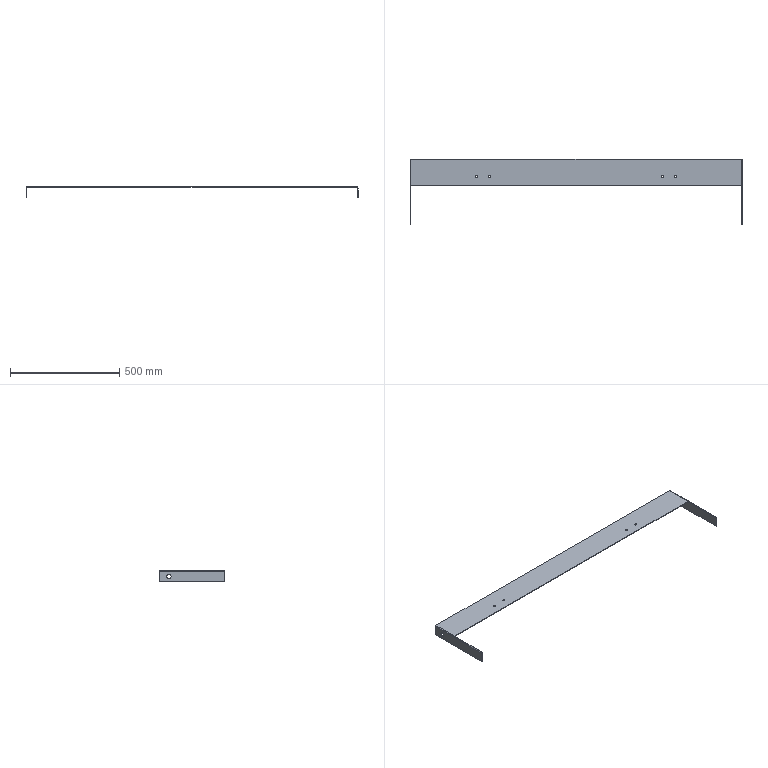Part | SolidWorks | features ICE 6, EdgeFlange 2, FlatPattern 1, MirrorPattern 1, SMBaseFlange 1, SheetMetal 1 | 1 solid | 36 faces | box 1518 x 301 x 50 mm | volume 631038 mm3 | plane 20 | cylinder 16 | commonest cylinder face diameters 9 x8 20 x4 1.473 x2 7.473 x2
STEP:
#1=CARTESIAN_POINT('',(450.763,220.,-3.));
#2=VERTEX_POINT('',#1);
#3=CARTESIAN_POINT('',(459.763,220.,-3.));
#4=VERTEX_POINT('',#3);
#5=CARTESIAN_POINT('',(455.263,220.,-3.));
#6=DIRECTION('',(0.,0.,1.));
#7=DIRECTION('',(-1.,0.,0.));
#8=AXIS2_PLACEMENT_3D('',#5,#6,#7);
#9=CIRCLE('',#8,4.5);
#10=EDGE_CURVE('',#2,#4,#9,.T.);
#11=ORIENTED_EDGE('',*,*,#10,.F.);
#12=CARTESIAN_POINT('',(450.763,220.,0.));
#13=VERTEX_POINT('',#12);
#14=CARTESIAN_POINT('',(450.763,220.,-50.));
#15=DIRECTION('',(0.,0.,1.));
#16=VECTOR('',#15,1000.);
#17=LINE('',#14,#16);
#18=EDGE_CURVE('',#2,#13,#17,.T.);
#19=ORIENTED_EDGE('',*,*,#18,.T.);
#20=CARTESIAN_POINT('',(459.763,220.,0.));
#21=VERTEX_POINT('',#20);
#22=CARTESIAN_POINT('',(455.263,220.,0.));
#23=DIRECTION('',(0.,0.,-1.));
#24=DIRECTION('',(-1.,0.,0.));
#25=AXIS2_PLACEMENT_3D('',#22,#23,#24);
#26=CIRCLE('',#25,4.5);
#27=EDGE_CURVE('',#21,#13,#26,.T.);
#28=ORIENTED_EDGE('',*,*,#27,.F.);
#29=CARTESIAN_POINT('',(459.763,220.,-50.));
#30=DIRECTION('',(0.,0.,1.));
#31=VECTOR('',#30,1000.);
#32=LINE('',#29,#31);
#33=EDGE_CURVE('',#4,#21,#32,.T.);
#34=ORIENTED_EDGE('',*,*,#33,.F.);
#35=EDGE_LOOP('',(#11,#19,#28,#34));
#36=FACE_OUTER_BOUND('',#35,.T.);
#37=CARTESIAN_POINT('',(455.263,220.,-50.));
#38=DIRECTION('',(0.,0.,1.));
#39=DIRECTION('',(1.,0.,0.));
#40=AXIS2_PLACEMENT_3D('',#37,#38,#39);
#41=CYLINDRICAL_SURFACE('',#40,4.5);
#42=ADVANCED_FACE('',(#36),#41,.F.);
#43=CARTESIAN_POINT('',(390.763,220.,-3.));
#44=VERTEX_POINT('',#43);
#45=CARTESIAN_POINT('',(399.763,220.,-3.));
#46=VERTEX_POINT('',#45);
#47=CARTESIAN_POINT('',(395.263,220.,-3.));
#48=DIRECTION('',(0.,0.,1.));
#49=DIRECTION('',(-1.,0.,0.));
#50=AXIS2_PLACEMENT_3D('',#47,#48,#49);
#51=CIRCLE('',#50,4.5);
#52=EDGE_CURVE('',#44,#46,#51,.T.);
#53=ORIENTED_EDGE('',*,*,#52,.F.);
#54=CARTESIAN_POINT('',(390.763,220.,0.));
#55=VERTEX_POINT('',#54);
#56=CARTESIAN_POINT('',(390.763,220.,-50.));
#57=DIRECTION('',(0.,0.,1.));
#58=VECTOR('',#57,1000.);
#59=LINE('',#56,#58);
#60=EDGE_CURVE('',#44,#55,#59,.T.);
#61=ORIENTED_EDGE('',*,*,#60,.T.);
#62=CARTESIAN_POINT('',(399.763,220.,0.));
#63=VERTEX_POINT('',#62);
#64=CARTESIAN_POINT('',(395.263,220.,0.));
#65=DIRECTION('',(0.,0.,1.));
#66=DIRECTION('',(-1.,0.,0.));
#67=AXIS2_PLACEMENT_3D('',#64,#65,#66);
#68=CIRCLE('',#67,4.5);
#69=EDGE_CURVE('',#55,#63,#68,.T.);
#70=ORIENTED_EDGE('',*,*,#69,.T.);
#71=CARTESIAN_POINT('',(399.763,220.,-50.));
#72=DIRECTION('',(0.,0.,1.));
#73=VECTOR('',#72,1000.);
#74=LINE('',#71,#73);
#75=EDGE_CURVE('',#46,#63,#74,.T.);
#76=ORIENTED_EDGE('',*,*,#75,.F.);
#77=EDGE_LOOP('',(#53,#61,#70,#76));
#78=FACE_OUTER_BOUND('',#77,.T.);
#79=CARTESIAN_POINT('',(395.263,220.,-50.));
#80=DIRECTION('',(0.,0.,1.));
#81=DIRECTION('',(1.,0.,0.));
#82=AXIS2_PLACEMENT_3D('',#79,#80,#81);
#83=CYLINDRICAL_SURFACE('',#82,4.5);
#84=ADVANCED_FACE('',(#78),#83,.F.);
#85=CARTESIAN_POINT('',(-450.763,220.,-3.));
#86=VERTEX_POINT('',#85);
#87=CARTESIAN_POINT('',(-459.763,220.,-3.));
#88=VERTEX_POINT('',#87);
#89=CARTESIAN_POINT('',(-455.263,220.,-3.));
#90=DIRECTION('',(0.,0.,-1.));
#91=DIRECTION('',(-1.,0.,0.));
#92=AXIS2_PLACEMENT_3D('',#89,#90,#91);
#93=CIRCLE('',#92,4.5);
#94=EDGE_CURVE('',#86,#88,#93,.T.);
#95=ORIENTED_EDGE('',*,*,#94,.T.);
#96=CARTESIAN_POINT('',(-459.763,220.,0.));
#97=VERTEX_POINT('',#96);
#98=CARTESIAN_POINT('',(-459.763,220.,-50.));
#99=DIRECTION('',(0.,0.,1.));
#100=VECTOR('',#99,1000.);
#101=LINE('',#98,#100);
#102=EDGE_CURVE('',#88,#97,#101,.T.);
#103=ORIENTED_EDGE('',*,*,#102,.T.);
#104=CARTESIAN_POINT('',(-450.763,220.,0.));
#105=VERTEX_POINT('',#104);
#106=CARTESIAN_POINT('',(-455.263,220.,0.));
#107=DIRECTION('',(0.,0.,1.));
#108=DIRECTION('',(1.,0.,0.));
#109=AXIS2_PLACEMENT_3D('',#106,#107,#108);
#110=CIRCLE('',#109,4.5);
#111=EDGE_CURVE('',#97,#105,#110,.T.);
#112=ORIENTED_EDGE('',*,*,#111,.T.);
#113=CARTESIAN_POINT('',(-450.763,220.,-50.));
#114=DIRECTION('',(0.,0.,1.));
#115=VECTOR('',#114,1000.);
#116=LINE('',#113,#115);
#117=EDGE_CURVE('',#86,#105,#116,.T.);
#118=ORIENTED_EDGE('',*,*,#117,.F.);
#119=EDGE_LOOP('',(#95,#103,#112,#118));
#120=FACE_OUTER_BOUND('',#119,.T.);
#121=CARTESIAN_POINT('',(-455.263,220.,-50.));
#122=DIRECTION('',(0.,0.,1.));
#123=DIRECTION('',(1.,0.,0.));
#124=AXIS2_PLACEMENT_3D('',#121,#122,#123);
#125=CYLINDRICAL_SURFACE('',#124,4.5);
#126=ADVANCED_FACE('',(#120),#125,.F.);
#127=CARTESIAN_POINT('',(-390.763,220.,-3.));
#128=VERTEX_POINT('',#127);
#129=CARTESIAN_POINT('',(-399.763,220.,-3.));
#130=VERTEX_POINT('',#129);
#131=CARTESIAN_POINT('',(-395.263,220.,-3.));
#132=DIRECTION('',(0.,0.,-1.));
#133=DIRECTION('',(-1.,0.,0.));
#134=AXIS2_PLACEMENT_3D('',#131,#132,#133);
#135=CIRCLE('',#134,4.5);
#136=EDGE_CURVE('',#128,#130,#135,.T.);
#137=ORIENTED_EDGE('',*,*,#136,.T.);
#138=CARTESIAN_POINT('',(-399.763,220.,0.));
#139=VERTEX_POINT('',#138);
#140=CARTESIAN_POINT('',(-399.763,220.,-50.));
#141=DIRECTION('',(0.,0.,1.));
#142=VECTOR('',#141,1000.);
#143=LINE('',#140,#142);
#144=EDGE_CURVE('',#130,#139,#143,.T.);
#145=ORIENTED_EDGE('',*,*,#144,.T.);
#146=CARTESIAN_POINT('',(-390.763,220.,0.));
#147=VERTEX_POINT('',#146);
#148=CARTESIAN_POINT('',(-395.263,220.,0.));
#149=DIRECTION('',(0.,0.,-1.));
#150=DIRECTION('',(-1.,0.,0.));
#151=AXIS2_PLACEMENT_3D('',#148,#149,#150);
#152=CIRCLE('',#151,4.5);
#153=EDGE_CURVE('',#147,#139,#152,.T.);
#154=ORIENTED_EDGE('',*,*,#153,.F.);
#155=CARTESIAN_POINT('',(-390.763,220.,-50.));
#156=DIRECTION('',(0.,0.,1.));
#157=VECTOR('',#156,1000.);
#158=LINE('',#155,#157);
#159=EDGE_CURVE('',#128,#147,#158,.T.);
#160=ORIENTED_EDGE('',*,*,#159,.F.);
#161=EDGE_LOOP('',(#137,#145,#154,#160));
#162=FACE_OUTER_BOUND('',#161,.T.);
#163=CARTESIAN_POINT('',(-395.263,220.,-50.));
#164=DIRECTION('',(0.,0.,1.));
#165=DIRECTION('',(1.,0.,0.));
#166=AXIS2_PLACEMENT_3D('',#163,#164,#165);
#167=CYLINDRICAL_SURFACE('',#166,4.5);
#168=ADVANCED_FACE('',(#162),#167,.F.);
#169=CARTESIAN_POINT('',(-759.,255.,-16.868));
#170=VERTEX_POINT('',#169);
#171=CARTESIAN_POINT('',(-759.,255.,-36.868));
#172=VERTEX_POINT('',#171);
#173=CARTESIAN_POINT('',(-759.,255.,-26.868));
#174=DIRECTION('',(1.,0.,0.));
#175=DIRECTION('',(0.,0.,-1.));
#176=AXIS2_PLACEMENT_3D('',#173,#174,#175);
#177=CIRCLE('',#176,10.);
#178=EDGE_CURVE('',#170,#172,#177,.T.);
#179=ORIENTED_EDGE('',*,*,#178,.F.);
#180=CARTESIAN_POINT('',(-756.,255.,-16.868));
#181=VERTEX_POINT('',#180);
#182=CARTESIAN_POINT('',(-759.,255.,-16.868));
#183=DIRECTION('',(1.,0.,0.));
#184=VECTOR('',#183,1000.);
#185=LINE('',#182,#184);
#186=EDGE_CURVE('',#170,#181,#185,.T.);
#187=ORIENTED_EDGE('',*,*,#186,.T.);
#188=CARTESIAN_POINT('',(-756.,255.,-36.868));
#189=VERTEX_POINT('',#188);
#190=CARTESIAN_POINT('',(-756.,255.,-26.868));
#191=DIRECTION('',(-1.,0.,0.));
#192=DIRECTION('',(0.,0.,1.));
#193=AXIS2_PLACEMENT_3D('',#190,#191,#192);
#194=CIRCLE('',#193,10.);
#195=EDGE_CURVE('',#189,#181,#194,.T.);
#196=ORIENTED_EDGE('',*,*,#195,.F.);
#197=CARTESIAN_POINT('',(-759.,255.,-36.868));
#198=DIRECTION('',(1.,0.,0.));
#199=VECTOR('',#198,1000.);
#200=LINE('',#197,#199);
#201=EDGE_CURVE('',#172,#189,#200,.T.);
#202=ORIENTED_EDGE('',*,*,#201,.F.);
#203=EDGE_LOOP('',(#179,#187,#196,#202));
#204=FACE_OUTER_BOUND('',#203,.T.);
#205=CARTESIAN_POINT('',(-759.,255.,-26.868));
#206=DIRECTION('',(1.,0.,0.));
#207=DIRECTION('',(0.,0.,-1.));
#208=AXIS2_PLACEMENT_3D('',#205,#206,#207);
#209=CYLINDRICAL_SURFACE('',#208,10.);
#210=ADVANCED_FACE('',(#204),#209,.F.);
#211=CARTESIAN_POINT('',(756.,255.,-16.868));
#212=VERTEX_POINT('',#211);
#213=CARTESIAN_POINT('',(756.,255.,-36.868));
#214=VERTEX_POINT('',#213);
#215=CARTESIAN_POINT('',(756.,255.,-26.868));
#216=DIRECTION('',(1.,0.,0.));
#217=DIRECTION('',(0.,0.,-1.));
#218=AXIS2_PLACEMENT_3D('',#215,#216,#217);
#219=CIRCLE('',#218,10.);
#220=EDGE_CURVE('',#212,#214,#219,.T.);
#221=ORIENTED_EDGE('',*,*,#220,.F.);
#222=CARTESIAN_POINT('',(759.,255.,-16.868));
#223=VERTEX_POINT('',#222);
#224=CARTESIAN_POINT('',(-759.,255.,-16.868));
#225=DIRECTION('',(1.,0.,0.));
#226=VECTOR('',#225,1000.);
#227=LINE('',#224,#226);
#228=EDGE_CURVE('',#212,#223,#227,.T.);
#229=ORIENTED_EDGE('',*,*,#228,.T.);
#230=CARTESIAN_POINT('',(759.,255.,-36.868));
#231=VERTEX_POINT('',#230);
#232=CARTESIAN_POINT('',(759.,255.,-26.868));
#233=DIRECTION('',(1.,0.,0.));
#234=DIRECTION('',(0.,0.,-1.));
#235=AXIS2_PLACEMENT_3D('',#232,#233,#234);
#236=CIRCLE('',#235,10.);
#237=EDGE_CURVE('',#223,#231,#236,.T.);
#238=ORIENTED_EDGE('',*,*,#237,.T.);
#239=CARTESIAN_POINT('',(-759.,255.,-36.868));
#240=DIRECTION('',(1.,0.,0.));
#241=VECTOR('',#240,1000.);
#242=LINE('',#239,#241);
#243=EDGE_CURVE('',#214,#231,#242,.T.);
#244=ORIENTED_EDGE('',*,*,#243,.F.);
#245=EDGE_LOOP('',(#221,#229,#238,#244));
#246=FACE_OUTER_BOUND('',#245,.T.);
#247=CARTESIAN_POINT('',(-759.,255.,-26.868));
#248=DIRECTION('',(1.,0.,0.));
#249=DIRECTION('',(0.,0.,-1.));
#250=AXIS2_PLACEMENT_3D('',#247,#248,#249);
#251=CYLINDRICAL_SURFACE('',#250,10.);
#252=ADVANCED_FACE('',(#246),#251,.F.);
#253=CARTESIAN_POINT('',(-756.,-1.,-3.737));
#254=VERTEX_POINT('',#253);
#255=CARTESIAN_POINT('',(-756.,-1.,-50.));
#256=VERTEX_POINT('',#255);
#257=CARTESIAN_POINT('',(-756.,-1.,0.));
#258=DIRECTION('',(0.,0.,-1.));
#259=VECTOR('',#258,1000.);
#260=LINE('',#257,#259);
#261=EDGE_CURVE('',#254,#256,#260,.T.);
#262=ORIENTED_EDGE('',*,*,#261,.F.);
#263=CARTESIAN_POINT('',(-759.,-1.,-3.737));
#264=VERTEX_POINT('',#263);
#265=CARTESIAN_POINT('',(-756.,-1.,-3.737));
#266=DIRECTION('',(-1.,0.,0.));
#267=VECTOR('',#266,1000.);
#268=LINE('',#265,#267);
#269=EDGE_CURVE('',#254,#264,#268,.T.);
#270=ORIENTED_EDGE('',*,*,#269,.T.);
#271=CARTESIAN_POINT('',(-759.,-1.,-50.));
#272=VERTEX_POINT('',#271);
#273=CARTESIAN_POINT('',(-759.,-1.,-141.819));
#274=DIRECTION('',(0.,0.,1.));
#275=VECTOR('',#274,1000.);
#276=LINE('',#273,#275);
#277=EDGE_CURVE('',#272,#264,#276,.T.);
#278=ORIENTED_EDGE('',*,*,#277,.F.);
#279=CARTESIAN_POINT('',(-759.,-1.,-50.));
#280=DIRECTION('',(1.,0.,0.));
#281=VECTOR('',#280,1000.);
#282=LINE('',#279,#281);
#283=EDGE_CURVE('',#272,#256,#282,.T.);
#284=ORIENTED_EDGE('',*,*,#283,.T.);
#285=EDGE_LOOP('',(#262,#270,#278,#284));
#286=FACE_OUTER_BOUND('',#285,.T.);
#287=CARTESIAN_POINT('',(-759.,-1.,-141.819));
#288=DIRECTION('',(0.,1.,0.));
#289=DIRECTION('',(0.,0.,1.));
#290=AXIS2_PLACEMENT_3D('',#287,#288,#289);
#291=PLANE('',#290);
#292=ADVANCED_FACE('',(#286),#291,.F.);
#293=CARTESIAN_POINT('',(759.,-1.,-50.));
#294=VERTEX_POINT('',#293);
#295=CARTESIAN_POINT('',(759.,-1.,-3.737));
#296=VERTEX_POINT('',#295);
#297=CARTESIAN_POINT('',(759.,-1.,0.));
#298=DIRECTION('',(0.,0.,1.));
#299=VECTOR('',#298,1000.);
#300=LINE('',#297,#299);
#301=EDGE_CURVE('',#294,#296,#300,.T.);
#302=ORIENTED_EDGE('',*,*,#301,.T.);
#303=CARTESIAN_POINT('',(756.,-1.,-3.737));
#304=VERTEX_POINT('',#303);
#305=CARTESIAN_POINT('',(759.,-1.,-3.737));
#306=DIRECTION('',(-1.,0.,0.));
#307=VECTOR('',#306,1000.);
#308=LINE('',#305,#307);
#309=EDGE_CURVE('',#296,#304,#308,.T.);
#310=ORIENTED_EDGE('',*,*,#309,.T.);
#311=CARTESIAN_POINT('',(756.,-1.,-50.));
#312=VERTEX_POINT('',#311);
#313=CARTESIAN_POINT('',(756.,-1.,0.));
#314=DIRECTION('',(0.,0.,1.));
#315=VECTOR('',#314,1000.);
#316=LINE('',#313,#315);
#317=EDGE_CURVE('',#312,#304,#316,.T.);
#318=ORIENTED_EDGE('',*,*,#317,.F.);
#319=CARTESIAN_POINT('',(759.,-1.,-50.));
#320=DIRECTION('',(1.,0.,0.));
#321=VECTOR('',#320,1000.);
#322=LINE('',#319,#321);
#323=EDGE_CURVE('',#312,#294,#322,.T.);
#324=ORIENTED_EDGE('',*,*,#323,.T.);
#325=EDGE_LOOP('',(#302,#310,#318,#324));
#326=FACE_OUTER_BOUND('',#325,.T.);
#327=CARTESIAN_POINT('',(-759.,-1.,-141.819));
#328=DIRECTION('',(0.,1.,0.));
#329=DIRECTION('',(0.,0.,1.));
#330=AXIS2_PLACEMENT_3D('',#327,#328,#329);
#331=PLANE('',#330);
#332=ADVANCED_FACE('',(#326),#331,.F.);
#333=CARTESIAN_POINT('',(455.263,220.,-3.));
#334=DIRECTION('',(0.,0.,1.));
#335=DIRECTION('',(-1.,0.,0.));
#336=AXIS2_PLACEMENT_3D('',#333,#334,#335);
#337=CIRCLE('',#336,4.5);
#338=EDGE_CURVE('',#4,#2,#337,.T.);
#339=ORIENTED_EDGE('',*,*,#338,.T.);
#340=ORIENTED_EDGE('',*,*,#10,.T.);
#341=EDGE_LOOP('',(#339,#340));
#342=FACE_BOUND('',#341,.T.);
#343=CARTESIAN_POINT('',(395.263,220.,-3.));
#344=DIRECTION('',(0.,0.,1.));
#345=DIRECTION('',(-1.,0.,0.));
#346=AXIS2_PLACEMENT_3D('',#343,#344,#345);
#347=CIRCLE('',#346,4.5);
#348=EDGE_CURVE('',#46,#44,#347,.T.);
#349=ORIENTED_EDGE('',*,*,#348,.T.);
#350=ORIENTED_EDGE('',*,*,#52,.T.);
#351=EDGE_LOOP('',(#349,#350));
#352=FACE_BOUND('',#351,.T.);
#353=ORIENTED_EDGE('',*,*,#94,.F.);
#354=CARTESIAN_POINT('',(-455.263,220.,-3.));
#355=DIRECTION('',(0.,0.,-1.));
#356=DIRECTION('',(-1.,0.,0.));
#357=AXIS2_PLACEMENT_3D('',#354,#355,#356);
#358=CIRCLE('',#357,4.5);
#359=EDGE_CURVE('',#88,#86,#358,.T.);
#360=ORIENTED_EDGE('',*,*,#359,.F.);
#361=EDGE_LOOP('',(#353,#360));
#362=FACE_BOUND('',#361,.T.);
#363=ORIENTED_EDGE('',*,*,#136,.F.);
#364=CARTESIAN_POINT('',(-395.263,220.,-3.));
#365=DIRECTION('',(0.,0.,-1.));
#366=DIRECTION('',(-1.,0.,0.));
#367=AXIS2_PLACEMENT_3D('',#364,#365,#366);
#368=CIRCLE('',#367,4.5);
#369=EDGE_CURVE('',#130,#128,#368,.T.);
#370=ORIENTED_EDGE('',*,*,#369,.F.);
#371=EDGE_LOOP('',(#363,#370));
#372=FACE_BOUND('',#371,.T.);
#373=CARTESIAN_POINT('',(-755.263,180.,-3.));
#374=VERTEX_POINT('',#373);
#375=CARTESIAN_POINT('',(755.263,180.,-3.));
#376=VERTEX_POINT('',#375);
#377=CARTESIAN_POINT('',(755.263,180.,-3.));
#378=DIRECTION('',(1.,0.,0.));
#379=VECTOR('',#378,1000.);
#380=LINE('',#377,#379);
#381=EDGE_CURVE('',#374,#376,#380,.T.);
#382=ORIENTED_EDGE('',*,*,#381,.F.);
#383=CARTESIAN_POINT('',(-755.263,300.,-3.));
#384=VERTEX_POINT('',#383);
#385=CARTESIAN_POINT('',(-755.263,300.,-3.));
#386=DIRECTION('',(0.,-1.,0.));
#387=VECTOR('',#386,1000.);
#388=LINE('',#385,#387);
#389=EDGE_CURVE('',#384,#374,#388,.T.);
#390=ORIENTED_EDGE('',*,*,#389,.F.);
#391=CARTESIAN_POINT('',(755.263,300.,-3.));
#392=VERTEX_POINT('',#391);
#393=CARTESIAN_POINT('',(-759.,300.,-3.));
#394=DIRECTION('',(-1.,0.,0.));
#395=VECTOR('',#394,1000.);
#396=LINE('',#393,#395);
#397=EDGE_CURVE('',#392,#384,#396,.T.);
#398=ORIENTED_EDGE('',*,*,#397,.F.);
#399=CARTESIAN_POINT('',(755.263,-300.,-3.));
#400=DIRECTION('',(0.,1.,0.));
#401=VECTOR('',#400,1000.);
#402=LINE('',#399,#401);
#403=EDGE_CURVE('',#376,#392,#402,.T.);
#404=ORIENTED_EDGE('',*,*,#403,.F.);
#405=EDGE_LOOP('',(#382,#390,#398,#404));
#406=FACE_OUTER_BOUND('',#405,.T.);
#407=CARTESIAN_POINT('',(0.,0.,-3.));
#408=DIRECTION('',(0.,0.,-1.));
#409=DIRECTION('',(-1.,0.,0.));
#410=AXIS2_PLACEMENT_3D('',#407,#408,#409);
#411=PLANE('',#410);
#412=ADVANCED_FACE('',(#342,#352,#362,#372,#406),#411,.T.);
#413=ORIENTED_EDGE('',*,*,#27,.T.);
#414=CARTESIAN_POINT('',(455.263,220.,0.));
#415=DIRECTION('',(0.,0.,-1.));
#416=DIRECTION('',(-1.,0.,0.));
#417=AXIS2_PLACEMENT_3D('',#414,#415,#416);
#418=CIRCLE('',#417,4.5);
#419=EDGE_CURVE('',#13,#21,#418,.T.);
#420=ORIENTED_EDGE('',*,*,#419,.T.);
#421=EDGE_LOOP('',(#413,#420));
#422=FACE_BOUND('',#421,.T.);
#423=CARTESIAN_POINT('',(395.263,220.,0.));
#424=DIRECTION('',(0.,0.,1.));
#425=DIRECTION('',(-1.,0.,0.));
#426=AXIS2_PLACEMENT_3D('',#423,#424,#425);
#427=CIRCLE('',#426,4.5);
#428=EDGE_CURVE('',#63,#55,#427,.T.);
#429=ORIENTED_EDGE('',*,*,#428,.F.);
#430=ORIENTED_EDGE('',*,*,#69,.F.);
#431=EDGE_LOOP('',(#429,#430));
#432=FACE_BOUND('',#431,.T.);
#433=CARTESIAN_POINT('',(-455.263,220.,0.));
#434=DIRECTION('',(0.,0.,1.));
#435=DIRECTION('',(1.,0.,0.));
#436=AXIS2_PLACEMENT_3D('',#433,#434,#435);
#437=CIRCLE('',#436,4.5);
#438=EDGE_CURVE('',#105,#97,#437,.T.);
#439=ORIENTED_EDGE('',*,*,#438,.F.);
#440=ORIENTED_EDGE('',*,*,#111,.F.);
#441=EDGE_LOOP('',(#439,#440));
#442=FACE_BOUND('',#441,.T.);
#443=ORIENTED_EDGE('',*,*,#153,.T.);
#444=CARTESIAN_POINT('',(-395.263,220.,0.));
#445=DIRECTION('',(0.,0.,-1.));
#446=DIRECTION('',(-1.,0.,0.));
#447=AXIS2_PLACEMENT_3D('',#444,#445,#446);
#448=CIRCLE('',#447,4.5);
#449=EDGE_CURVE('',#139,#147,#448,.T.);
#450=ORIENTED_EDGE('',*,*,#449,.T.);
#451=EDGE_LOOP('',(#443,#450));
#452=FACE_BOUND('',#451,.T.);
#453=CARTESIAN_POINT('',(-755.263,300.,0.));
#454=VERTEX_POINT('',#453);
#455=CARTESIAN_POINT('',(-755.263,180.,0.));
#456=VERTEX_POINT('',#455);
#457=CARTESIAN_POINT('',(-755.263,300.,0.));
#458=DIRECTION('',(0.,-1.,0.));
#459=VECTOR('',#458,1000.);
#460=LINE('',#457,#459);
#461=EDGE_CURVE('',#454,#456,#460,.T.);
#462=ORIENTED_EDGE('',*,*,#461,.T.);
#463=CARTESIAN_POINT('',(755.263,180.,0.));
#464=VERTEX_POINT('',#463);
#465=CARTESIAN_POINT('',(755.263,180.,0.));
#466=DIRECTION('',(1.,0.,0.));
#467=VECTOR('',#466,1000.);
#468=LINE('',#465,#467);
#469=EDGE_CURVE('',#456,#464,#468,.T.);
#470=ORIENTED_EDGE('',*,*,#469,.T.);
#471=CARTESIAN_POINT('',(755.263,300.,0.));
#472=VERTEX_POINT('',#471);
#473=CARTESIAN_POINT('',(755.263,-300.,0.));
#474=DIRECTION('',(0.,1.,0.));
#475=VECTOR('',#474,1000.);
#476=LINE('',#473,#475);
#477=EDGE_CURVE('',#464,#472,#476,.T.);
#478=ORIENTED_EDGE('',*,*,#477,.T.);
#479=CARTESIAN_POINT('',(-759.,300.,0.));
#480=DIRECTION('',(-1.,0.,0.));
#481=VECTOR('',#480,1000.);
#482=LINE('',#479,#481);
#483=EDGE_CURVE('',#472,#454,#482,.T.);
#484=ORIENTED_EDGE('',*,*,#483,.T.);
#485=EDGE_LOOP('',(#462,#470,#478,#484));
#486=FACE_OUTER_BOUND('',#485,.T.);
#487=CARTESIAN_POINT('',(0.,0.,0.));
#488=DIRECTION('',(0.,0.,-1.));
#489=DIRECTION('',(-1.,0.,0.));
#490=AXIS2_PLACEMENT_3D('',#487,#488,#489);
#491=PLANE('',#490);
#492=ADVANCED_FACE('',(#422,#432,#442,#452,#486),#491,.F.);
#493=CARTESIAN_POINT('',(755.263,300.,-3.));
#494=DIRECTION('',(0.,0.,1.));
#495=VECTOR('',#494,1000.);
#496=LINE('',#493,#495);
#497=EDGE_CURVE('',#392,#472,#496,.T.);
#498=ORIENTED_EDGE('',*,*,#497,.F.);
#499=ORIENTED_EDGE('',*,*,#397,.T.);
#500=CARTESIAN_POINT('',(-755.263,300.,-3.));
#501=DIRECTION('',(0.,0.,1.));
#502=VECTOR('',#501,1000.);
#503=LINE('',#500,#502);
#504=EDGE_CURVE('',#384,#454,#503,.T.);
#505=ORIENTED_EDGE('',*,*,#504,.T.);
#506=ORIENTED_EDGE('',*,*,#483,.F.);
#507=EDGE_LOOP('',(#498,#499,#505,#506));
#508=FACE_OUTER_BOUND('',#507,.T.);
#509=CARTESIAN_POINT('',(-759.,300.,-3.));
#510=DIRECTION('',(0.,1.,0.));
#511=DIRECTION('',(0.,0.,1.));
#512=AXIS2_PLACEMENT_3D('',#509,#510,#511);
#513=PLANE('',#512);
#514=ADVANCED_FACE('',(#508),#513,.T.);
#515=CARTESIAN_POINT('',(-756.,300.,-3.737));
#516=VERTEX_POINT('',#515);
#517=CARTESIAN_POINT('',(-755.263,300.,-3.737));
#518=DIRECTION('',(0.,1.,0.));
#519=DIRECTION('',(0.,0.,1.));
#520=AXIS2_PLACEMENT_3D('',#517,#518,#519);
#521=CIRCLE('',#520,0.7366);
#522=EDGE_CURVE('',#516,#384,#521,.T.);
#523=ORIENTED_EDGE('',*,*,#522,.F.);
#524=CARTESIAN_POINT('',(-759.,300.,-3.737));
#525=VERTEX_POINT('',#524);
#526=CARTESIAN_POINT('',(-756.,300.,-3.737));
#527=DIRECTION('',(-1.,0.,0.));
#528=VECTOR('',#527,1000.);
#529=LINE('',#526,#528);
#530=EDGE_CURVE('',#516,#525,#529,.T.);
#531=ORIENTED_EDGE('',*,*,#530,.T.);
#532=CARTESIAN_POINT('',(-755.263,300.,-3.737));
#533=DIRECTION('',(0.,1.,0.));
#534=DIRECTION('',(0.,0.,1.));
#535=AXIS2_PLACEMENT_3D('',#532,#533,#534);
#536=CIRCLE('',#535,3.737);
#537=EDGE_CURVE('',#525,#454,#536,.T.);
#538=ORIENTED_EDGE('',*,*,#537,.T.);
#539=ORIENTED_EDGE('',*,*,#504,.F.);
#540=EDGE_LOOP('',(#523,#531,#538,#539));
#541=FACE_OUTER_BOUND('',#540,.T.);
#542=CARTESIAN_POINT('',(-755.263,300.,-3.737));
#543=DIRECTION('',(0.,-1.,0.));
#544=DIRECTION('',(0.,0.,-1.));
#545=AXIS2_PLACEMENT_3D('',#542,#543,#544);
#546=PLANE('',#545);
#547=ADVANCED_FACE('',(#541),#546,.F.);
#548=CARTESIAN_POINT('',(-755.263,-1.,0.));
#549=VERTEX_POINT('',#548);
#550=CARTESIAN_POINT('',(-755.263,-1.,-3.737));
#551=DIRECTION('',(0.,-1.,0.));
#552=DIRECTION('',(0.,0.,1.));
#553=AXIS2_PLACEMENT_3D('',#550,#551,#552);
#554=CIRCLE('',#553,3.737);
#555=EDGE_CURVE('',#549,#264,#554,.T.);
#556=ORIENTED_EDGE('',*,*,#555,.F.);
#557=CARTESIAN_POINT('',(-755.263,300.,0.));
#558=DIRECTION('',(0.,-1.,0.));
#559=VECTOR('',#558,1000.);
#560=LINE('',#557,#559);
#561=EDGE_CURVE('',#456,#549,#560,.T.);
#562=ORIENTED_EDGE('',*,*,#561,.F.);
#563=ORIENTED_EDGE('',*,*,#461,.F.);
#564=ORIENTED_EDGE('',*,*,#537,.F.);
#565=CARTESIAN_POINT('',(-759.,0.,-3.737));
#566=DIRECTION('',(0.,1.,0.));
#567=VECTOR('',#566,1000.);
#568=LINE('',#565,#567);
#569=EDGE_CURVE('',#264,#525,#568,.T.);
#570=ORIENTED_EDGE('',*,*,#569,.F.);
#571=EDGE_LOOP('',(#556,#562,#563,#564,#570));
#572=FACE_OUTER_BOUND('',#571,.T.);
#573=CARTESIAN_POINT('',(-755.263,300.,-3.737));
#574=DIRECTION('',(0.,1.,0.));
#575=DIRECTION('',(-1.,0.,0.));
#576=AXIS2_PLACEMENT_3D('',#573,#574,#575);
#577=CYLINDRICAL_SURFACE('',#576,3.737);
#578=ADVANCED_FACE('',(#572),#577,.T.);
#579=CARTESIAN_POINT('',(-755.263,-1.,-3.));
#580=VERTEX_POINT('',#579);
#581=CARTESIAN_POINT('',(-755.263,300.,-3.));
#582=DIRECTION('',(0.,-1.,0.));
#583=VECTOR('',#582,1000.);
#584=LINE('',#581,#583);
#585=EDGE_CURVE('',#374,#580,#584,.T.);
#586=ORIENTED_EDGE('',*,*,#585,.T.);
#587=CARTESIAN_POINT('',(-755.263,-1.,-3.737));
#588=DIRECTION('',(0.,-1.,0.));
#589=DIRECTION('',(0.,0.,1.));
#590=AXIS2_PLACEMENT_3D('',#587,#588,#589);
#591=CIRCLE('',#590,0.7366);
#592=EDGE_CURVE('',#580,#254,#591,.T.);
#593=ORIENTED_EDGE('',*,*,#592,.T.);
#594=CARTESIAN_POINT('',(-756.,-300.,-3.737));
#595=DIRECTION('',(0.,1.,0.));
#596=VECTOR('',#595,1000.);
#597=LINE('',#594,#596);
#598=EDGE_CURVE('',#254,#516,#597,.T.);
#599=ORIENTED_EDGE('',*,*,#598,.T.);
#600=ORIENTED_EDGE('',*,*,#522,.T.);
#601=ORIENTED_EDGE('',*,*,#389,.T.);
#602=EDGE_LOOP('',(#586,#593,#599,#600,#601));
#603=FACE_OUTER_BOUND('',#602,.T.);
#604=CARTESIAN_POINT('',(-755.263,300.,-3.737));
#605=DIRECTION('',(0.,1.,0.));
#606=DIRECTION('',(-1.,0.,0.));
#607=AXIS2_PLACEMENT_3D('',#604,#605,#606);
#608=CYLINDRICAL_SURFACE('',#607,0.7366);
#609=ADVANCED_FACE('',(#603),#608,.F.);
#610=CARTESIAN_POINT('',(-759.,300.,-50.));
#611=VERTEX_POINT('',#610);
#612=CARTESIAN_POINT('',(-759.,300.,-3.));
#613=DIRECTION('',(0.,0.,1.));
#614=VECTOR('',#613,1000.);
#615=LINE('',#612,#614);
#616=EDGE_CURVE('',#611,#525,#615,.T.);
#617=ORIENTED_EDGE('',*,*,#616,.T.);
#618=ORIENTED_EDGE('',*,*,#530,.F.);
#619=CARTESIAN_POINT('',(-756.,300.,-50.));
#620=VERTEX_POINT('',#619);
#621=CARTESIAN_POINT('',(-756.,300.,0.));
#622=DIRECTION('',(0.,0.,1.));
#623=VECTOR('',#622,1000.);
#624=LINE('',#621,#623);
#625=EDGE_CURVE('',#620,#516,#624,.T.);
#626=ORIENTED_EDGE('',*,*,#625,.F.);
#627=CARTESIAN_POINT('',(-759.,300.,-50.));
#628=DIRECTION('',(1.,0.,0.));
#629=VECTOR('',#628,1000.);
#630=LINE('',#627,#629);
#631=EDGE_CURVE('',#611,#620,#630,.T.);
#632=ORIENTED_EDGE('',*,*,#631,.F.);
#633=EDGE_LOOP('',(#617,#618,#626,#632));
#634=FACE_OUTER_BOUND('',#633,.T.);
#635=CARTESIAN_POINT('',(-759.,300.,-3.));
#636=DIRECTION('',(0.,1.,0.));
#637=DIRECTION('',(0.,0.,1.));
#638=AXIS2_PLACEMENT_3D('',#635,#636,#637);
#639=PLANE('',#638);
#640=ADVANCED_FACE('',(#634),#639,.T.);
#641=ORIENTED_EDGE('',*,*,#277,.T.);
#642=ORIENTED_EDGE('',*,*,#569,.T.);
#643=ORIENTED_EDGE('',*,*,#616,.F.);
#644=CARTESIAN_POINT('',(-759.,300.,-50.));
#645=DIRECTION('',(0.,1.,0.));
#646=VECTOR('',#645,1000.);
#647=LINE('',#644,#646);
#648=EDGE_CURVE('',#272,#611,#647,.T.);
#649=ORIENTED_EDGE('',*,*,#648,.F.);
#650=EDGE_LOOP('',(#641,#642,#643,#649));
#651=FACE_OUTER_BOUND('',#650,.T.);
#652=CARTESIAN_POINT('',(-759.,255.,-26.868));
#653=DIRECTION('',(1.,0.,0.));
#654=DIRECTION('',(0.,0.,-1.));
#655=AXIS2_PLACEMENT_3D('',#652,#653,#654);
#656=CIRCLE('',#655,10.);
#657=EDGE_CURVE('',#172,#170,#656,.T.);
#658=ORIENTED_EDGE('',*,*,#657,.T.);
#659=ORIENTED_EDGE('',*,*,#178,.T.);
#660=EDGE_LOOP('',(#658,#659));
#661=FACE_BOUND('',#660,.T.);
#662=CARTESIAN_POINT('',(-759.,0.,0.));
#663=DIRECTION('',(-1.,0.,0.));
#664=DIRECTION('',(0.,0.,1.));
#665=AXIS2_PLACEMENT_3D('',#662,#663,#664);
#666=PLANE('',#665);
#667=ADVANCED_FACE('',(#651,#661),#666,.T.);
#668=ORIENTED_EDGE('',*,*,#195,.T.);
#669=CARTESIAN_POINT('',(-756.,255.,-26.868));
#670=DIRECTION('',(-1.,0.,0.));
#671=DIRECTION('',(0.,0.,1.));
#672=AXIS2_PLACEMENT_3D('',#669,#670,#671);
#673=CIRCLE('',#672,10.);
#674=EDGE_CURVE('',#181,#189,#673,.T.);
#675=ORIENTED_EDGE('',*,*,#674,.T.);
#676=EDGE_LOOP('',(#668,#675));
#677=FACE_BOUND('',#676,.T.);
#678=ORIENTED_EDGE('',*,*,#598,.F.);
#679=ORIENTED_EDGE('',*,*,#261,.T.);
#680=CARTESIAN_POINT('',(-756.,0.,-50.));
#681=DIRECTION('',(0.,1.,0.));
#682=VECTOR('',#681,1000.);
#683=LINE('',#680,#682);
#684=EDGE_CURVE('',#256,#620,#683,.T.);
#685=ORIENTED_EDGE('',*,*,#684,.T.);
#686=ORIENTED_EDGE('',*,*,#625,.T.);
#687=EDGE_LOOP('',(#678,#679,#685,#686));
#688=FACE_OUTER_BOUND('',#687,.T.);
#689=CARTESIAN_POINT('',(-756.,0.,0.));
#690=DIRECTION('',(-1.,0.,0.));
#691=DIRECTION('',(0.,0.,1.));
#692=AXIS2_PLACEMENT_3D('',#689,#690,#691);
#693=PLANE('',#692);
#694=ADVANCED_FACE('',(#677,#688),#693,.F.);
#695=ORIENTED_EDGE('',*,*,#283,.F.);
#696=ORIENTED_EDGE('',*,*,#648,.T.);
#697=ORIENTED_EDGE('',*,*,#631,.T.);
#698=ORIENTED_EDGE('',*,*,#684,.F.);
#699=EDGE_LOOP('',(#695,#696,#697,#698));
#700=FACE_OUTER_BOUND('',#699,.T.);
#701=CARTESIAN_POINT('',(-759.,300.,-50.));
#702=DIRECTION('',(0.,0.,-1.));
#703=DIRECTION('',(-1.,0.,0.));
#704=AXIS2_PLACEMENT_3D('',#701,#702,#703);
#705=PLANE('',#704);
#706=ADVANCED_FACE('',(#700),#705,.T.);
#707=CARTESIAN_POINT('',(756.,300.,-3.737));
#708=VERTEX_POINT('',#707);
#709=CARTESIAN_POINT('',(759.,300.,-3.737));
#710=VERTEX_POINT('',#709);
#711=CARTESIAN_POINT('',(759.,300.,-3.737));
#712=DIRECTION('',(1.,0.,0.));
#713=VECTOR('',#712,1000.);
#714=LINE('',#711,#713);
#715=EDGE_CURVE('',#708,#710,#714,.T.);
#716=ORIENTED_EDGE('',*,*,#715,.F.);
#717=CARTESIAN_POINT('',(755.263,300.,-3.737));
#718=DIRECTION('',(0.,1.,0.));
#719=DIRECTION('',(0.,0.,-1.));
#720=AXIS2_PLACEMENT_3D('',#717,#718,#719);
#721=CIRCLE('',#720,0.7366);
#722=EDGE_CURVE('',#392,#708,#721,.T.);
#723=ORIENTED_EDGE('',*,*,#722,.F.);
#724=ORIENTED_EDGE('',*,*,#497,.T.);
#725=CARTESIAN_POINT('',(755.263,300.,-3.737));
#726=DIRECTION('',(0.,1.,0.));
#727=DIRECTION('',(0.,0.,-1.));
#728=AXIS2_PLACEMENT_3D('',#725,#726,#727);
#729=CIRCLE('',#728,3.737);
#730=EDGE_CURVE('',#472,#710,#729,.T.);
#731=ORIENTED_EDGE('',*,*,#730,.T.);
#732=EDGE_LOOP('',(#716,#723,#724,#731));
#733=FACE_OUTER_BOUND('',#732,.T.);
#734=CARTESIAN_POINT('',(755.263,300.,-3.737));
#735=DIRECTION('',(0.,1.,0.));
#736=DIRECTION('',(0.,0.,1.));
#737=AXIS2_PLACEMENT_3D('',#734,#735,#736);
#738=PLANE('',#737);
#739=ADVANCED_FACE('',(#733),#738,.T.);
#740=CARTESIAN_POINT('',(755.263,-1.,0.));
#741=VERTEX_POINT('',#740);
#742=CARTESIAN_POINT('',(755.263,-1.,-3.737));
#743=DIRECTION('',(0.,-1.,0.));
#744=DIRECTION('',(0.,0.,1.));
#745=AXIS2_PLACEMENT_3D('',#742,#743,#744);
#746=CIRCLE('',#745,3.737);
#747=EDGE_CURVE('',#296,#741,#746,.T.);
#748=ORIENTED_EDGE('',*,*,#747,.F.);
#749=CARTESIAN_POINT('',(759.,0.,-3.737));
#750=DIRECTION('',(0.,-1.,0.));
#751=VECTOR('',#750,1000.);
#752=LINE('',#749,#751);
#753=EDGE_CURVE('',#710,#296,#752,.T.);
#754=ORIENTED_EDGE('',*,*,#753,.F.);
#755=ORIENTED_EDGE('',*,*,#730,.F.);
#756=ORIENTED_EDGE('',*,*,#477,.F.);
#757=CARTESIAN_POINT('',(755.263,-300.,0.));
#758=DIRECTION('',(0.,1.,0.));
#759=VECTOR('',#758,1000.);
#760=LINE('',#757,#759);
#761=EDGE_CURVE('',#741,#464,#760,.T.);
#762=ORIENTED_EDGE('',*,*,#761,.F.);
#763=EDGE_LOOP('',(#748,#754,#755,#756,#762));
#764=FACE_OUTER_BOUND('',#763,.T.);
#765=CARTESIAN_POINT('',(755.263,-300.,-3.737));
#766=DIRECTION('',(0.,-1.,0.));
#767=DIRECTION('',(1.,0.,0.));
#768=AXIS2_PLACEMENT_3D('',#765,#766,#767);
#769=CYLINDRICAL_SURFACE('',#768,3.737);
#770=ADVANCED_FACE('',(#764),#769,.T.);
#771=CARTESIAN_POINT('',(756.,300.,-3.737));
#772=DIRECTION('',(0.,-1.,0.));
#773=VECTOR('',#772,1000.);
#774=LINE('',#771,#773);
#775=EDGE_CURVE('',#708,#304,#774,.T.);
#776=ORIENTED_EDGE('',*,*,#775,.T.);
#777=CARTESIAN_POINT('',(755.263,-1.,-3.));
#778=VERTEX_POINT('',#777);
#779=CARTESIAN_POINT('',(755.263,-1.,-3.737));
#780=DIRECTION('',(0.,-1.,0.));
#781=DIRECTION('',(0.,0.,1.));
#782=AXIS2_PLACEMENT_3D('',#779,#780,#781);
#783=CIRCLE('',#782,0.7366);
#784=EDGE_CURVE('',#304,#778,#783,.T.);
#785=ORIENTED_EDGE('',*,*,#784,.T.);
#786=CARTESIAN_POINT('',(755.263,-300.,-3.));
#787=DIRECTION('',(0.,1.,0.));
#788=VECTOR('',#787,1000.);
#789=LINE('',#786,#788);
#790=EDGE_CURVE('',#778,#376,#789,.T.);
#791=ORIENTED_EDGE('',*,*,#790,.T.);
#792=ORIENTED_EDGE('',*,*,#403,.T.);
#793=ORIENTED_EDGE('',*,*,#722,.T.);
#794=EDGE_LOOP('',(#776,#785,#791,#792,#793));
#795=FACE_OUTER_BOUND('',#794,.T.);
#796=CARTESIAN_POINT('',(755.263,-300.,-3.737));
#797=DIRECTION('',(0.,-1.,0.));
#798=DIRECTION('',(1.,0.,0.));
#799=AXIS2_PLACEMENT_3D('',#796,#797,#798);
#800=CYLINDRICAL_SURFACE('',#799,0.7366);
#801=ADVANCED_FACE('',(#795),#800,.F.);
#802=CARTESIAN_POINT('',(756.,300.,-50.));
#803=VERTEX_POINT('',#802);
#804=CARTESIAN_POINT('',(756.,300.,0.));
#805=DIRECTION('',(0.,0.,-1.));
#806=VECTOR('',#805,1000.);
#807=LINE('',#804,#806);
#808=EDGE_CURVE('',#708,#803,#807,.T.);
#809=ORIENTED_EDGE('',*,*,#808,.F.);
#810=ORIENTED_EDGE('',*,*,#715,.T.);
#811=CARTESIAN_POINT('',(759.,300.,-50.));
#812=VERTEX_POINT('',#811);
#813=CARTESIAN_POINT('',(759.,300.,-50.));
#814=DIRECTION('',(0.,0.,-1.));
#815=VECTOR('',#814,1000.);
#816=LINE('',#813,#815);
#817=EDGE_CURVE('',#710,#812,#816,.T.);
#818=ORIENTED_EDGE('',*,*,#817,.T.);
#819=CARTESIAN_POINT('',(759.,300.,-50.));
#820=DIRECTION('',(-1.,0.,0.));
#821=VECTOR('',#820,1000.);
#822=LINE('',#819,#821);
#823=EDGE_CURVE('',#812,#803,#822,.T.);
#824=ORIENTED_EDGE('',*,*,#823,.T.);
#825=EDGE_LOOP('',(#809,#810,#818,#824));
#826=FACE_OUTER_BOUND('',#825,.T.);
#827=CARTESIAN_POINT('',(759.,300.,-50.));
#828=DIRECTION('',(0.,1.,0.));
#829=DIRECTION('',(0.,0.,1.));
#830=AXIS2_PLACEMENT_3D('',#827,#828,#829);
#831=PLANE('',#830);
#832=ADVANCED_FACE('',(#826),#831,.T.);
#833=ORIENTED_EDGE('',*,*,#301,.F.);
#834=CARTESIAN_POINT('',(759.,-300.,-50.));
#835=DIRECTION('',(0.,-1.,0.));
#836=VECTOR('',#835,1000.);
#837=LINE('',#834,#836);
#838=EDGE_CURVE('',#812,#294,#837,.T.);
#839=ORIENTED_EDGE('',*,*,#838,.F.);
#840=ORIENTED_EDGE('',*,*,#817,.F.);
#841=ORIENTED_EDGE('',*,*,#753,.T.);
#842=EDGE_LOOP('',(#833,#839,#840,#841));
#843=FACE_OUTER_BOUND('',#842,.T.);
#844=CARTESIAN_POINT('',(759.,255.,-26.868));
#845=DIRECTION('',(1.,0.,0.));
#846=DIRECTION('',(0.,0.,-1.));
#847=AXIS2_PLACEMENT_3D('',#844,#845,#846);
#848=CIRCLE('',#847,10.);
#849=EDGE_CURVE('',#231,#223,#848,.T.);
#850=ORIENTED_EDGE('',*,*,#849,.F.);
#851=ORIENTED_EDGE('',*,*,#237,.F.);
#852=EDGE_LOOP('',(#850,#851));
#853=FACE_BOUND('',#852,.T.);
#854=CARTESIAN_POINT('',(759.,0.,0.));
#855=DIRECTION('',(1.,0.,0.));
#856=DIRECTION('',(0.,0.,-1.));
#857=AXIS2_PLACEMENT_3D('',#854,#855,#856);
#858=PLANE('',#857);
#859=ADVANCED_FACE('',(#843,#853),#858,.T.);
#860=CARTESIAN_POINT('',(756.,255.,-26.868));
#861=DIRECTION('',(1.,0.,0.));
#862=DIRECTION('',(0.,0.,-1.));
#863=AXIS2_PLACEMENT_3D('',#860,#861,#862);
#864=CIRCLE('',#863,10.);
#865=EDGE_CURVE('',#214,#212,#864,.T.);
#866=ORIENTED_EDGE('',*,*,#865,.T.);
#867=ORIENTED_EDGE('',*,*,#220,.T.);
#868=EDGE_LOOP('',(#866,#867));
#869=FACE_BOUND('',#868,.T.);
#870=CARTESIAN_POINT('',(756.,0.,-50.));
#871=DIRECTION('',(0.,-1.,0.));
#872=VECTOR('',#871,1000.);
#873=LINE('',#870,#872);
#874=EDGE_CURVE('',#803,#312,#873,.T.);
#875=ORIENTED_EDGE('',*,*,#874,.T.);
#876=ORIENTED_EDGE('',*,*,#317,.T.);
#877=ORIENTED_EDGE('',*,*,#775,.F.);
#878=ORIENTED_EDGE('',*,*,#808,.T.);
#879=EDGE_LOOP('',(#875,#876,#877,#878));
#880=FACE_OUTER_BOUND('',#879,.T.);
#881=CARTESIAN_POINT('',(756.,0.,0.));
#882=DIRECTION('',(1.,0.,0.));
#883=DIRECTION('',(0.,0.,-1.));
#884=AXIS2_PLACEMENT_3D('',#881,#882,#883);
#885=PLANE('',#884);
#886=ADVANCED_FACE('',(#869,#880),#885,.F.);
#887=ORIENTED_EDGE('',*,*,#323,.F.);
#888=ORIENTED_EDGE('',*,*,#874,.F.);
#889=ORIENTED_EDGE('',*,*,#823,.F.);
#890=ORIENTED_EDGE('',*,*,#838,.T.);
#891=EDGE_LOOP('',(#887,#888,#889,#890));
#892=FACE_OUTER_BOUND('',#891,.T.);
#893=CARTESIAN_POINT('',(759.,-300.,-50.));
#894=DIRECTION('',(0.,0.,-1.));
#895=DIRECTION('',(-1.,0.,0.));
#896=AXIS2_PLACEMENT_3D('',#893,#894,#895);
#897=PLANE('',#896);
#898=ADVANCED_FACE('',(#892),#897,.T.);
#899=ORIENTED_EDGE('',*,*,#228,.F.);
#900=ORIENTED_EDGE('',*,*,#865,.F.);
#901=ORIENTED_EDGE('',*,*,#243,.T.);
#902=ORIENTED_EDGE('',*,*,#849,.T.);
#903=EDGE_LOOP('',(#899,#900,#901,#902));
#904=FACE_OUTER_BOUND('',#903,.T.);
#905=CARTESIAN_POINT('',(-759.,255.,-26.868));
#906=DIRECTION('',(1.,0.,0.));
#907=DIRECTION('',(0.,0.,-1.));
#908=AXIS2_PLACEMENT_3D('',#905,#906,#907);
#909=CYLINDRICAL_SURFACE('',#908,10.);
#910=ADVANCED_FACE('',(#904),#909,.F.);
#911=ORIENTED_EDGE('',*,*,#186,.F.);
#912=ORIENTED_EDGE('',*,*,#657,.F.);
#913=ORIENTED_EDGE('',*,*,#201,.T.);
#914=ORIENTED_EDGE('',*,*,#674,.F.);
#915=EDGE_LOOP('',(#911,#912,#913,#914));
#916=FACE_OUTER_BOUND('',#915,.T.);
#917=CARTESIAN_POINT('',(-759.,255.,-26.868));
#918=DIRECTION('',(1.,0.,0.));
#919=DIRECTION('',(0.,0.,-1.));
#920=AXIS2_PLACEMENT_3D('',#917,#918,#919);
#921=CYLINDRICAL_SURFACE('',#920,10.);
#922=ADVANCED_FACE('',(#916),#921,.F.);
#923=ORIENTED_EDGE('',*,*,#561,.T.);
#924=CARTESIAN_POINT('',(-755.263,-1.,0.));
#925=DIRECTION('',(0.,0.,-1.));
#926=VECTOR('',#925,1000.);
#927=LINE('',#924,#926);
#928=EDGE_CURVE('',#549,#580,#927,.T.);
#929=ORIENTED_EDGE('',*,*,#928,.T.);
#930=ORIENTED_EDGE('',*,*,#585,.F.);
#931=CARTESIAN_POINT('',(-755.263,180.,0.));
#932=DIRECTION('',(0.,0.,-1.));
#933=VECTOR('',#932,1000.);
#934=LINE('',#931,#933);
#935=EDGE_CURVE('',#456,#374,#934,.T.);
#936=ORIENTED_EDGE('',*,*,#935,.F.);
#937=EDGE_LOOP('',(#923,#929,#930,#936));
#938=FACE_OUTER_BOUND('',#937,.T.);
#939=CARTESIAN_POINT('',(-755.263,180.,0.));
#940=DIRECTION('',(-1.,0.,0.));
#941=DIRECTION('',(0.,0.,1.));
#942=AXIS2_PLACEMENT_3D('',#939,#940,#941);
#943=PLANE('',#942);
#944=ADVANCED_FACE('',(#938),#943,.F.);
#945=ORIENTED_EDGE('',*,*,#790,.F.);
#946=CARTESIAN_POINT('',(755.263,-1.,0.));
#947=DIRECTION('',(0.,0.,1.));
#948=VECTOR('',#947,1000.);
#949=LINE('',#946,#948);
#950=EDGE_CURVE('',#778,#741,#949,.T.);
#951=ORIENTED_EDGE('',*,*,#950,.T.);
#952=ORIENTED_EDGE('',*,*,#761,.T.);
#953=CARTESIAN_POINT('',(755.263,180.,0.));
#954=DIRECTION('',(0.,0.,-1.));
#955=VECTOR('',#954,1000.);
#956=LINE('',#953,#955);
#957=EDGE_CURVE('',#464,#376,#956,.T.);
#958=ORIENTED_EDGE('',*,*,#957,.T.);
#959=EDGE_LOOP('',(#945,#951,#952,#958));
#960=FACE_OUTER_BOUND('',#959,.T.);
#961=CARTESIAN_POINT('',(755.263,180.,0.));
#962=DIRECTION('',(1.,0.,0.));
#963=DIRECTION('',(0.,0.,-1.));
#964=AXIS2_PLACEMENT_3D('',#961,#962,#963);
#965=PLANE('',#964);
#966=ADVANCED_FACE('',(#960),#965,.F.);
#967=ORIENTED_EDGE('',*,*,#381,.T.);
#968=ORIENTED_EDGE('',*,*,#957,.F.);
#969=ORIENTED_EDGE('',*,*,#469,.F.);
#970=ORIENTED_EDGE('',*,*,#935,.T.);
#971=EDGE_LOOP('',(#967,#968,#969,#970));
#972=FACE_OUTER_BOUND('',#971,.T.);
#973=CARTESIAN_POINT('',(755.263,180.,0.));
#974=DIRECTION('',(0.,1.,0.));
#975=DIRECTION('',(0.,0.,1.));
#976=AXIS2_PLACEMENT_3D('',#973,#974,#975);
#977=PLANE('',#976);
#978=ADVANCED_FACE('',(#972),#977,.F.);
#979=ORIENTED_EDGE('',*,*,#144,.F.);
#980=ORIENTED_EDGE('',*,*,#369,.T.);
#981=ORIENTED_EDGE('',*,*,#159,.T.);
#982=ORIENTED_EDGE('',*,*,#449,.F.);
#983=EDGE_LOOP('',(#979,#980,#981,#982));
#984=FACE_OUTER_BOUND('',#983,.T.);
#985=CARTESIAN_POINT('',(-395.263,220.,-50.));
#986=DIRECTION('',(0.,0.,1.));
#987=DIRECTION('',(1.,0.,0.));
#988=AXIS2_PLACEMENT_3D('',#985,#986,#987);
#989=CYLINDRICAL_SURFACE('',#988,4.5);
#990=ADVANCED_FACE('',(#984),#989,.F.);
#991=ORIENTED_EDGE('',*,*,#309,.F.);
#992=ORIENTED_EDGE('',*,*,#747,.T.);
#993=ORIENTED_EDGE('',*,*,#950,.F.);
#994=ORIENTED_EDGE('',*,*,#784,.F.);
#995=EDGE_LOOP('',(#991,#992,#993,#994));
#996=FACE_OUTER_BOUND('',#995,.T.);
#997=CARTESIAN_POINT('',(-759.,-1.,-141.819));
#998=DIRECTION('',(0.,1.,0.));
#999=DIRECTION('',(0.,0.,1.));
#1000=AXIS2_PLACEMENT_3D('',#997,#998,#999);
#1001=PLANE('',#1000);
#1002=ADVANCED_FACE('',(#996),#1001,.F.);
#1003=ORIENTED_EDGE('',*,*,#269,.F.);
#1004=ORIENTED_EDGE('',*,*,#592,.F.);
#1005=ORIENTED_EDGE('',*,*,#928,.F.);
#1006=ORIENTED_EDGE('',*,*,#555,.T.);
#1007=EDGE_LOOP('',(#1003,#1004,#1005,#1006));
#1008=FACE_OUTER_BOUND('',#1007,.T.);
#1009=CARTESIAN_POINT('',(-759.,-1.,-141.819));
#1010=DIRECTION('',(0.,1.,0.));
#1011=DIRECTION('',(0.,0.,1.));
#1012=AXIS2_PLACEMENT_3D('',#1009,#1010,#1011);
#1013=PLANE('',#1012);
#1014=ADVANCED_FACE('',(#1008),#1013,.F.);
#1015=ORIENTED_EDGE('',*,*,#102,.F.);
#1016=ORIENTED_EDGE('',*,*,#359,.T.);
#1017=ORIENTED_EDGE('',*,*,#117,.T.);
#1018=ORIENTED_EDGE('',*,*,#438,.T.);
#1019=EDGE_LOOP('',(#1015,#1016,#1017,#1018));
#1020=FACE_OUTER_BOUND('',#1019,.T.);
#1021=CARTESIAN_POINT('',(-455.263,220.,-50.));
#1022=DIRECTION('',(0.,0.,1.));
#1023=DIRECTION('',(1.,0.,0.));
#1024=AXIS2_PLACEMENT_3D('',#1021,#1022,#1023);
#1025=CYLINDRICAL_SURFACE('',#1024,4.5);
#1026=ADVANCED_FACE('',(#1020),#1025,.F.);
#1027=ORIENTED_EDGE('',*,*,#60,.F.);
#1028=ORIENTED_EDGE('',*,*,#348,.F.);
#1029=ORIENTED_EDGE('',*,*,#75,.T.);
#1030=ORIENTED_EDGE('',*,*,#428,.T.);
#1031=EDGE_LOOP('',(#1027,#1028,#1029,#1030));
#1032=FACE_OUTER_BOUND('',#1031,.T.);
#1033=CARTESIAN_POINT('',(395.263,220.,-50.));
#1034=DIRECTION('',(0.,0.,1.));
#1035=DIRECTION('',(1.,0.,0.));
#1036=AXIS2_PLACEMENT_3D('',#1033,#1034,#1035);
#1037=CYLINDRICAL_SURFACE('',#1036,4.5);
#1038=ADVANCED_FACE('',(#1032),#1037,.F.);
#1039=ORIENTED_EDGE('',*,*,#18,.F.);
#1040=ORIENTED_EDGE('',*,*,#338,.F.);
#1041=ORIENTED_EDGE('',*,*,#33,.T.);
#1042=ORIENTED_EDGE('',*,*,#419,.F.);
#1043=EDGE_LOOP('',(#1039,#1040,#1041,#1042));
#1044=FACE_OUTER_BOUND('',#1043,.T.);
#1045=CARTESIAN_POINT('',(455.263,220.,-50.));
#1046=DIRECTION('',(0.,0.,1.));
#1047=DIRECTION('',(1.,0.,0.));
#1048=AXIS2_PLACEMENT_3D('',#1045,#1046,#1047);
#1049=CYLINDRICAL_SURFACE('',#1048,4.5);
#1050=ADVANCED_FACE('',(#1044),#1049,.F.);
#1051=CLOSED_SHELL('',(#42,#84,#126,#168,#210,#252,#292,#332,#412,#492,#514,#547,#578,#609,#640,#667,#694,#706,#739,#770,#801,#832,#859,#886,#898,#910,#922,#944,#966,#978,#990,#1002,#1014,#1026,#1038,#1050));
#1052=MANIFOLD_SOLID_BREP('',#1051);
#1053=CARTESIAN_POINT('',(0.,0.,0.));
#1054=DIRECTION('',(0.,0.,1.));
#1055=DIRECTION('',(1.,0.,0.));
#1056=AXIS2_PLACEMENT_3D('',#1053,#1054,#1055);
#1057=(LENGTH_UNIT()NAMED_UNIT(*)SI_UNIT(.MILLI.,.METRE.));
#1058=UNCERTAINTY_MEASURE_WITH_UNIT(LENGTH_MEASURE(0.00001),#1057,'','');
#1059=(NAMED_UNIT(*)PLANE_ANGLE_UNIT()SI_UNIT($,.RADIAN.));
#1060=(NAMED_UNIT(*)SI_UNIT($,.STERADIAN.)SOLID_ANGLE_UNIT());
#1061=(GEOMETRIC_REPRESENTATION_CONTEXT(3)GLOBAL_UNCERTAINTY_ASSIGNED_CONTEXT((#1058))GLOBAL_UNIT_ASSIGNED_CONTEXT((#1057,#1059,#1060))REPRESENTATION_CONTEXT('',''));
#1062=ADVANCED_BREP_SHAPE_REPRESENTATION('',(#1052,#1056),#1061);